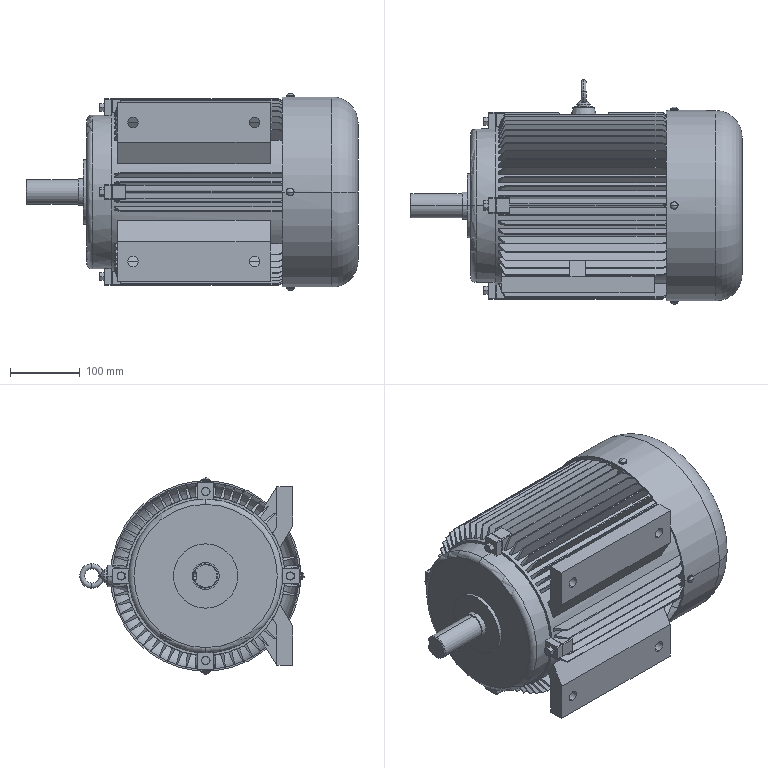Part | Creo | features COORDINATE SYSTEM 1, IMPORT FEATURE 1 | 1 solid | 540 faces | box 477.5 x 323.125 x 283.75 mm | volume 16550696 mm3 | plane 322 | cone 138 | cylinder 60 | torus 12 | sphere 8 | commonest cylinder face diameters 8.75 x8 10.25 x8 11.25 x8 15 x8 228.75 x8 268.75 x4